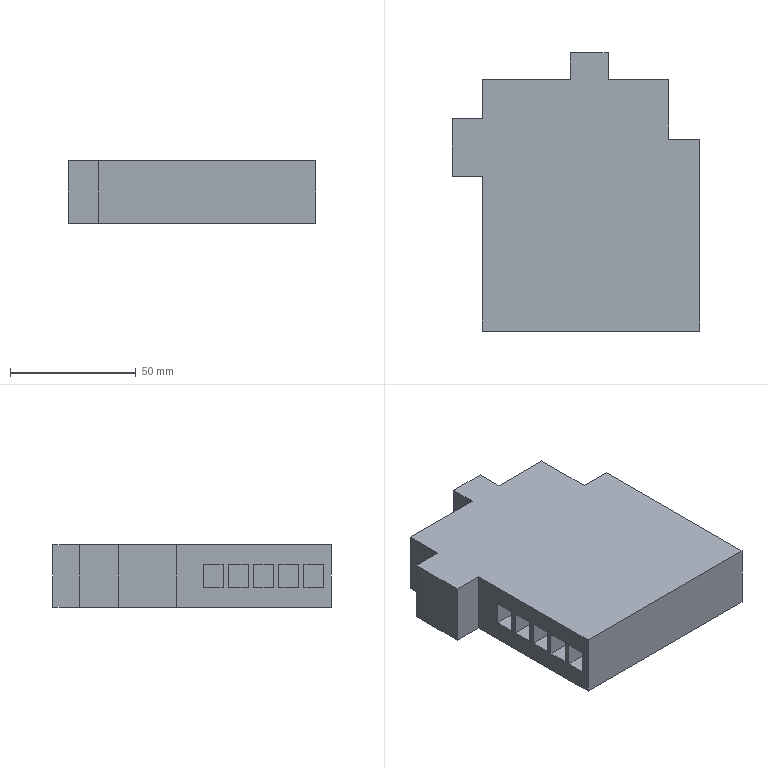Part | STEP file | 5-port DIN-rail switch EDS-205 | 1 solid | 41 faces | box 98.5 x 110.5 x 24.9 mm | volume 215104 mm3 | plane 41